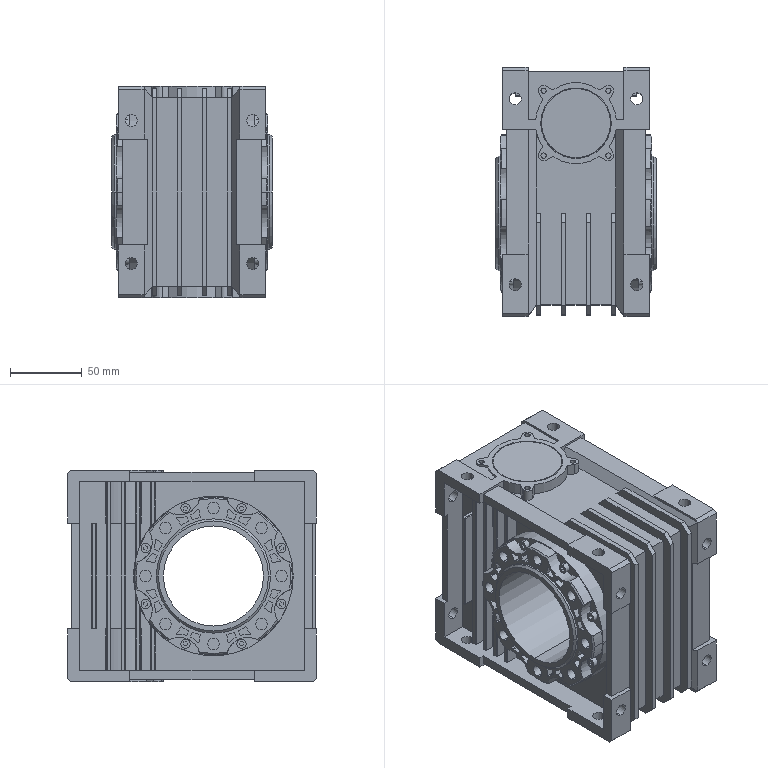Part | STEP file | RV025-090_063.step_1 | 1 solid | 863 faces | box 112 x 174 x 148 mm | volume 1644542 mm3 | plane 484 | cylinder 356 | cone 23 | commonest cylinder face diameters 1 x80 33.066 x36 6.5 x32 8 x32 8.5 x32 84 x32